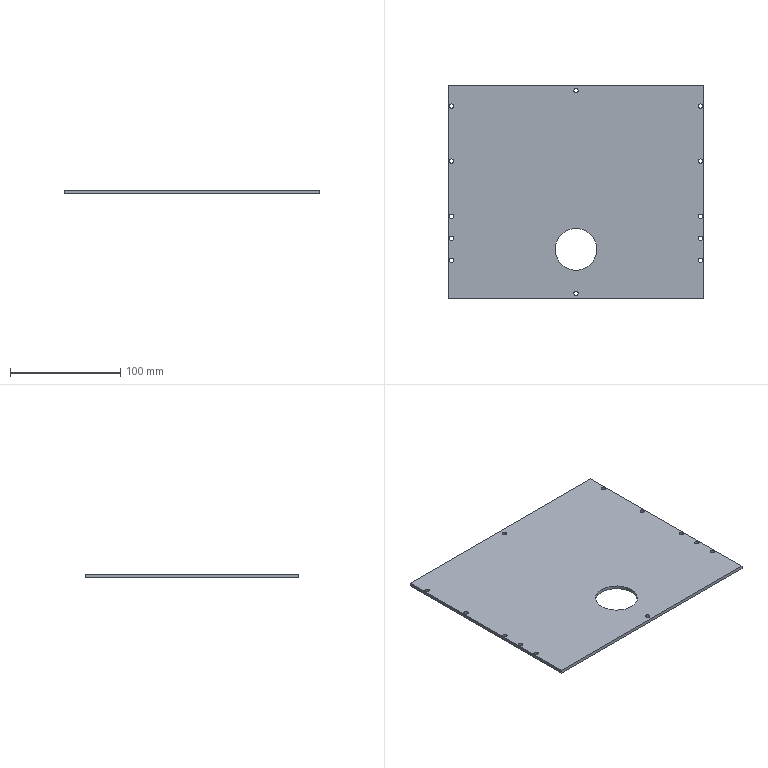Part | SolidWorks | features ICE 3, Extrusion 1, MirrorPattern 1 | 1 solid | 32 faces | box 232.3 x 194 x 3 mm | volume 131344 mm3 | cylinder 26 | plane 6 | commonest cylinder face diameters 4 x24 38 x2
STEP:
#1=CARTESIAN_POINT('',(115.15,-62.,0.));
#2=VERTEX_POINT('',#1);
#3=CARTESIAN_POINT('',(111.15,-62.,0.));
#4=VERTEX_POINT('',#3);
#5=CARTESIAN_POINT('',(113.15,-62.,0.));
#6=DIRECTION('',(0.,0.,-1.));
#7=DIRECTION('',(-1.,0.,0.));
#8=AXIS2_PLACEMENT_3D('',#5,#6,#7);
#9=CIRCLE('',#8,2.);
#10=EDGE_CURVE('',#2,#4,#9,.T.);
#11=ORIENTED_EDGE('',*,*,#10,.T.);
#12=CARTESIAN_POINT('',(111.15,-62.,3.));
#13=VERTEX_POINT('',#12);
#14=CARTESIAN_POINT('',(111.15,-62.,0.));
#15=DIRECTION('',(0.,0.,1.));
#16=VECTOR('',#15,1000.);
#17=LINE('',#14,#16);
#18=EDGE_CURVE('',#4,#13,#17,.T.);
#19=ORIENTED_EDGE('',*,*,#18,.T.);
#20=CARTESIAN_POINT('',(115.15,-62.,3.));
#21=VERTEX_POINT('',#20);
#22=CARTESIAN_POINT('',(113.15,-62.,3.));
#23=DIRECTION('',(0.,0.,-1.));
#24=DIRECTION('',(-1.,0.,0.));
#25=AXIS2_PLACEMENT_3D('',#22,#23,#24);
#26=CIRCLE('',#25,2.);
#27=EDGE_CURVE('',#21,#13,#26,.T.);
#28=ORIENTED_EDGE('',*,*,#27,.F.);
#29=CARTESIAN_POINT('',(115.15,-62.,0.));
#30=DIRECTION('',(0.,0.,1.));
#31=VECTOR('',#30,1000.);
#32=LINE('',#29,#31);
#33=EDGE_CURVE('',#2,#21,#32,.T.);
#34=ORIENTED_EDGE('',*,*,#33,.F.);
#35=EDGE_LOOP('',(#11,#19,#28,#34));
#36=FACE_OUTER_BOUND('',#35,.T.);
#37=CARTESIAN_POINT('',(113.15,-62.,0.));
#38=DIRECTION('',(0.,0.,1.));
#39=DIRECTION('',(1.,0.,0.));
#40=AXIS2_PLACEMENT_3D('',#37,#38,#39);
#41=CYLINDRICAL_SURFACE('',#40,2.);
#42=ADVANCED_FACE('',(#36),#41,.F.);
#43=CARTESIAN_POINT('',(115.15,-42.,0.));
#44=VERTEX_POINT('',#43);
#45=CARTESIAN_POINT('',(111.15,-42.,0.));
#46=VERTEX_POINT('',#45);
#47=CARTESIAN_POINT('',(113.15,-42.,0.));
#48=DIRECTION('',(0.,0.,-1.));
#49=DIRECTION('',(-1.,0.,0.));
#50=AXIS2_PLACEMENT_3D('',#47,#48,#49);
#51=CIRCLE('',#50,2.);
#52=EDGE_CURVE('',#44,#46,#51,.T.);
#53=ORIENTED_EDGE('',*,*,#52,.T.);
#54=CARTESIAN_POINT('',(111.15,-42.,3.));
#55=VERTEX_POINT('',#54);
#56=CARTESIAN_POINT('',(111.15,-42.,0.));
#57=DIRECTION('',(0.,0.,1.));
#58=VECTOR('',#57,1000.);
#59=LINE('',#56,#58);
#60=EDGE_CURVE('',#46,#55,#59,.T.);
#61=ORIENTED_EDGE('',*,*,#60,.T.);
#62=CARTESIAN_POINT('',(115.15,-42.,3.));
#63=VERTEX_POINT('',#62);
#64=CARTESIAN_POINT('',(113.15,-42.,3.));
#65=DIRECTION('',(0.,0.,-1.));
#66=DIRECTION('',(-1.,0.,0.));
#67=AXIS2_PLACEMENT_3D('',#64,#65,#66);
#68=CIRCLE('',#67,2.);
#69=EDGE_CURVE('',#63,#55,#68,.T.);
#70=ORIENTED_EDGE('',*,*,#69,.F.);
#71=CARTESIAN_POINT('',(115.15,-42.,0.));
#72=DIRECTION('',(0.,0.,1.));
#73=VECTOR('',#72,1000.);
#74=LINE('',#71,#73);
#75=EDGE_CURVE('',#44,#63,#74,.T.);
#76=ORIENTED_EDGE('',*,*,#75,.F.);
#77=EDGE_LOOP('',(#53,#61,#70,#76));
#78=FACE_OUTER_BOUND('',#77,.T.);
#79=CARTESIAN_POINT('',(113.15,-42.,0.));
#80=DIRECTION('',(0.,0.,1.));
#81=DIRECTION('',(1.,0.,0.));
#82=AXIS2_PLACEMENT_3D('',#79,#80,#81);
#83=CYLINDRICAL_SURFACE('',#82,2.);
#84=ADVANCED_FACE('',(#78),#83,.F.);
#85=CARTESIAN_POINT('',(115.15,-22.,0.));
#86=VERTEX_POINT('',#85);
#87=CARTESIAN_POINT('',(111.15,-22.,0.));
#88=VERTEX_POINT('',#87);
#89=CARTESIAN_POINT('',(113.15,-22.,0.));
#90=DIRECTION('',(0.,0.,-1.));
#91=DIRECTION('',(-1.,0.,0.));
#92=AXIS2_PLACEMENT_3D('',#89,#90,#91);
#93=CIRCLE('',#92,2.);
#94=EDGE_CURVE('',#86,#88,#93,.T.);
#95=ORIENTED_EDGE('',*,*,#94,.T.);
#96=CARTESIAN_POINT('',(111.15,-22.,3.));
#97=VERTEX_POINT('',#96);
#98=CARTESIAN_POINT('',(111.15,-22.,0.));
#99=DIRECTION('',(0.,0.,1.));
#100=VECTOR('',#99,1000.);
#101=LINE('',#98,#100);
#102=EDGE_CURVE('',#88,#97,#101,.T.);
#103=ORIENTED_EDGE('',*,*,#102,.T.);
#104=CARTESIAN_POINT('',(115.15,-22.,3.));
#105=VERTEX_POINT('',#104);
#106=CARTESIAN_POINT('',(113.15,-22.,3.));
#107=DIRECTION('',(0.,0.,-1.));
#108=DIRECTION('',(-1.,0.,0.));
#109=AXIS2_PLACEMENT_3D('',#106,#107,#108);
#110=CIRCLE('',#109,2.);
#111=EDGE_CURVE('',#105,#97,#110,.T.);
#112=ORIENTED_EDGE('',*,*,#111,.F.);
#113=CARTESIAN_POINT('',(115.15,-22.,0.));
#114=DIRECTION('',(0.,0.,1.));
#115=VECTOR('',#114,1000.);
#116=LINE('',#113,#115);
#117=EDGE_CURVE('',#86,#105,#116,.T.);
#118=ORIENTED_EDGE('',*,*,#117,.F.);
#119=EDGE_LOOP('',(#95,#103,#112,#118));
#120=FACE_OUTER_BOUND('',#119,.T.);
#121=CARTESIAN_POINT('',(113.15,-22.,0.));
#122=DIRECTION('',(0.,0.,1.));
#123=DIRECTION('',(1.,0.,0.));
#124=AXIS2_PLACEMENT_3D('',#121,#122,#123);
#125=CYLINDRICAL_SURFACE('',#124,2.);
#126=ADVANCED_FACE('',(#120),#125,.F.);
#127=CARTESIAN_POINT('',(115.15,28.,0.));
#128=VERTEX_POINT('',#127);
#129=CARTESIAN_POINT('',(111.15,28.,0.));
#130=VERTEX_POINT('',#129);
#131=CARTESIAN_POINT('',(113.15,28.,0.));
#132=DIRECTION('',(0.,0.,-1.));
#133=DIRECTION('',(-1.,0.,0.));
#134=AXIS2_PLACEMENT_3D('',#131,#132,#133);
#135=CIRCLE('',#134,2.);
#136=EDGE_CURVE('',#128,#130,#135,.T.);
#137=ORIENTED_EDGE('',*,*,#136,.T.);
#138=CARTESIAN_POINT('',(111.15,28.,3.));
#139=VERTEX_POINT('',#138);
#140=CARTESIAN_POINT('',(111.15,28.,0.));
#141=DIRECTION('',(0.,0.,1.));
#142=VECTOR('',#141,1000.);
#143=LINE('',#140,#142);
#144=EDGE_CURVE('',#130,#139,#143,.T.);
#145=ORIENTED_EDGE('',*,*,#144,.T.);
#146=CARTESIAN_POINT('',(115.15,28.,3.));
#147=VERTEX_POINT('',#146);
#148=CARTESIAN_POINT('',(113.15,28.,3.));
#149=DIRECTION('',(0.,0.,-1.));
#150=DIRECTION('',(-1.,0.,0.));
#151=AXIS2_PLACEMENT_3D('',#148,#149,#150);
#152=CIRCLE('',#151,2.);
#153=EDGE_CURVE('',#147,#139,#152,.T.);
#154=ORIENTED_EDGE('',*,*,#153,.F.);
#155=CARTESIAN_POINT('',(115.15,28.,0.));
#156=DIRECTION('',(0.,0.,1.));
#157=VECTOR('',#156,1000.);
#158=LINE('',#155,#157);
#159=EDGE_CURVE('',#128,#147,#158,.T.);
#160=ORIENTED_EDGE('',*,*,#159,.F.);
#161=EDGE_LOOP('',(#137,#145,#154,#160));
#162=FACE_OUTER_BOUND('',#161,.T.);
#163=CARTESIAN_POINT('',(113.15,28.,0.));
#164=DIRECTION('',(0.,0.,1.));
#165=DIRECTION('',(1.,0.,0.));
#166=AXIS2_PLACEMENT_3D('',#163,#164,#165);
#167=CYLINDRICAL_SURFACE('',#166,2.);
#168=ADVANCED_FACE('',(#162),#167,.F.);
#169=CARTESIAN_POINT('',(115.15,78.,0.));
#170=VERTEX_POINT('',#169);
#171=CARTESIAN_POINT('',(111.15,78.,0.));
#172=VERTEX_POINT('',#171);
#173=CARTESIAN_POINT('',(113.15,78.,0.));
#174=DIRECTION('',(0.,0.,-1.));
#175=DIRECTION('',(-1.,0.,0.));
#176=AXIS2_PLACEMENT_3D('',#173,#174,#175);
#177=CIRCLE('',#176,2.);
#178=EDGE_CURVE('',#170,#172,#177,.T.);
#179=ORIENTED_EDGE('',*,*,#178,.T.);
#180=CARTESIAN_POINT('',(111.15,78.,3.));
#181=VERTEX_POINT('',#180);
#182=CARTESIAN_POINT('',(111.15,78.,0.));
#183=DIRECTION('',(0.,0.,1.));
#184=VECTOR('',#183,1000.);
#185=LINE('',#182,#184);
#186=EDGE_CURVE('',#172,#181,#185,.T.);
#187=ORIENTED_EDGE('',*,*,#186,.T.);
#188=CARTESIAN_POINT('',(115.15,78.,3.));
#189=VERTEX_POINT('',#188);
#190=CARTESIAN_POINT('',(113.15,78.,3.));
#191=DIRECTION('',(0.,0.,-1.));
#192=DIRECTION('',(-1.,0.,0.));
#193=AXIS2_PLACEMENT_3D('',#190,#191,#192);
#194=CIRCLE('',#193,2.);
#195=EDGE_CURVE('',#189,#181,#194,.T.);
#196=ORIENTED_EDGE('',*,*,#195,.F.);
#197=CARTESIAN_POINT('',(115.15,78.,0.));
#198=DIRECTION('',(0.,0.,1.));
#199=VECTOR('',#198,1000.);
#200=LINE('',#197,#199);
#201=EDGE_CURVE('',#170,#189,#200,.T.);
#202=ORIENTED_EDGE('',*,*,#201,.F.);
#203=EDGE_LOOP('',(#179,#187,#196,#202));
#204=FACE_OUTER_BOUND('',#203,.T.);
#205=CARTESIAN_POINT('',(113.15,78.,0.));
#206=DIRECTION('',(0.,0.,1.));
#207=DIRECTION('',(1.,0.,0.));
#208=AXIS2_PLACEMENT_3D('',#205,#206,#207);
#209=CYLINDRICAL_SURFACE('',#208,2.);
#210=ADVANCED_FACE('',(#204),#209,.F.);
#211=CARTESIAN_POINT('',(-115.15,-62.,0.));
#212=VERTEX_POINT('',#211);
#213=CARTESIAN_POINT('',(-111.15,-62.,0.));
#214=VERTEX_POINT('',#213);
#215=CARTESIAN_POINT('',(-113.15,-62.,0.));
#216=DIRECTION('',(0.,0.,1.));
#217=DIRECTION('',(1.,0.,0.));
#218=AXIS2_PLACEMENT_3D('',#215,#216,#217);
#219=CIRCLE('',#218,2.);
#220=EDGE_CURVE('',#212,#214,#219,.T.);
#221=ORIENTED_EDGE('',*,*,#220,.F.);
#222=CARTESIAN_POINT('',(-115.15,-62.,3.));
#223=VERTEX_POINT('',#222);
#224=CARTESIAN_POINT('',(-115.15,-62.,0.));
#225=DIRECTION('',(0.,0.,1.));
#226=VECTOR('',#225,1000.);
#227=LINE('',#224,#226);
#228=EDGE_CURVE('',#212,#223,#227,.T.);
#229=ORIENTED_EDGE('',*,*,#228,.T.);
#230=CARTESIAN_POINT('',(-111.15,-62.,3.));
#231=VERTEX_POINT('',#230);
#232=CARTESIAN_POINT('',(-113.15,-62.,3.));
#233=DIRECTION('',(0.,0.,1.));
#234=DIRECTION('',(1.,0.,0.));
#235=AXIS2_PLACEMENT_3D('',#232,#233,#234);
#236=CIRCLE('',#235,2.);
#237=EDGE_CURVE('',#223,#231,#236,.T.);
#238=ORIENTED_EDGE('',*,*,#237,.T.);
#239=CARTESIAN_POINT('',(-111.15,-62.,0.));
#240=DIRECTION('',(0.,0.,1.));
#241=VECTOR('',#240,1000.);
#242=LINE('',#239,#241);
#243=EDGE_CURVE('',#214,#231,#242,.T.);
#244=ORIENTED_EDGE('',*,*,#243,.F.);
#245=EDGE_LOOP('',(#221,#229,#238,#244));
#246=FACE_OUTER_BOUND('',#245,.T.);
#247=CARTESIAN_POINT('',(-113.15,-62.,0.));
#248=DIRECTION('',(0.,0.,1.));
#249=DIRECTION('',(1.,0.,0.));
#250=AXIS2_PLACEMENT_3D('',#247,#248,#249);
#251=CYLINDRICAL_SURFACE('',#250,2.);
#252=ADVANCED_FACE('',(#246),#251,.F.);
#253=CARTESIAN_POINT('',(-115.15,-42.,0.));
#254=VERTEX_POINT('',#253);
#255=CARTESIAN_POINT('',(-111.15,-42.,0.));
#256=VERTEX_POINT('',#255);
#257=CARTESIAN_POINT('',(-113.15,-42.,0.));
#258=DIRECTION('',(0.,0.,1.));
#259=DIRECTION('',(1.,0.,0.));
#260=AXIS2_PLACEMENT_3D('',#257,#258,#259);
#261=CIRCLE('',#260,2.);
#262=EDGE_CURVE('',#254,#256,#261,.T.);
#263=ORIENTED_EDGE('',*,*,#262,.F.);
#264=CARTESIAN_POINT('',(-115.15,-42.,3.));
#265=VERTEX_POINT('',#264);
#266=CARTESIAN_POINT('',(-115.15,-42.,0.));
#267=DIRECTION('',(0.,0.,1.));
#268=VECTOR('',#267,1000.);
#269=LINE('',#266,#268);
#270=EDGE_CURVE('',#254,#265,#269,.T.);
#271=ORIENTED_EDGE('',*,*,#270,.T.);
#272=CARTESIAN_POINT('',(-111.15,-42.,3.));
#273=VERTEX_POINT('',#272);
#274=CARTESIAN_POINT('',(-113.15,-42.,3.));
#275=DIRECTION('',(0.,0.,1.));
#276=DIRECTION('',(1.,0.,0.));
#277=AXIS2_PLACEMENT_3D('',#274,#275,#276);
#278=CIRCLE('',#277,2.);
#279=EDGE_CURVE('',#265,#273,#278,.T.);
#280=ORIENTED_EDGE('',*,*,#279,.T.);
#281=CARTESIAN_POINT('',(-111.15,-42.,0.));
#282=DIRECTION('',(0.,0.,1.));
#283=VECTOR('',#282,1000.);
#284=LINE('',#281,#283);
#285=EDGE_CURVE('',#256,#273,#284,.T.);
#286=ORIENTED_EDGE('',*,*,#285,.F.);
#287=EDGE_LOOP('',(#263,#271,#280,#286));
#288=FACE_OUTER_BOUND('',#287,.T.);
#289=CARTESIAN_POINT('',(-113.15,-42.,0.));
#290=DIRECTION('',(0.,0.,1.));
#291=DIRECTION('',(1.,0.,0.));
#292=AXIS2_PLACEMENT_3D('',#289,#290,#291);
#293=CYLINDRICAL_SURFACE('',#292,2.);
#294=ADVANCED_FACE('',(#288),#293,.F.);
#295=CARTESIAN_POINT('',(-115.15,-22.,0.));
#296=VERTEX_POINT('',#295);
#297=CARTESIAN_POINT('',(-111.15,-22.,0.));
#298=VERTEX_POINT('',#297);
#299=CARTESIAN_POINT('',(-113.15,-22.,0.));
#300=DIRECTION('',(0.,0.,1.));
#301=DIRECTION('',(1.,0.,0.));
#302=AXIS2_PLACEMENT_3D('',#299,#300,#301);
#303=CIRCLE('',#302,2.);
#304=EDGE_CURVE('',#296,#298,#303,.T.);
#305=ORIENTED_EDGE('',*,*,#304,.F.);
#306=CARTESIAN_POINT('',(-115.15,-22.,3.));
#307=VERTEX_POINT('',#306);
#308=CARTESIAN_POINT('',(-115.15,-22.,0.));
#309=DIRECTION('',(0.,0.,1.));
#310=VECTOR('',#309,1000.);
#311=LINE('',#308,#310);
#312=EDGE_CURVE('',#296,#307,#311,.T.);
#313=ORIENTED_EDGE('',*,*,#312,.T.);
#314=CARTESIAN_POINT('',(-111.15,-22.,3.));
#315=VERTEX_POINT('',#314);
#316=CARTESIAN_POINT('',(-113.15,-22.,3.));
#317=DIRECTION('',(0.,0.,1.));
#318=DIRECTION('',(1.,0.,0.));
#319=AXIS2_PLACEMENT_3D('',#316,#317,#318);
#320=CIRCLE('',#319,2.);
#321=EDGE_CURVE('',#307,#315,#320,.T.);
#322=ORIENTED_EDGE('',*,*,#321,.T.);
#323=CARTESIAN_POINT('',(-111.15,-22.,0.));
#324=DIRECTION('',(0.,0.,1.));
#325=VECTOR('',#324,1000.);
#326=LINE('',#323,#325);
#327=EDGE_CURVE('',#298,#315,#326,.T.);
#328=ORIENTED_EDGE('',*,*,#327,.F.);
#329=EDGE_LOOP('',(#305,#313,#322,#328));
#330=FACE_OUTER_BOUND('',#329,.T.);
#331=CARTESIAN_POINT('',(-113.15,-22.,0.));
#332=DIRECTION('',(0.,0.,1.));
#333=DIRECTION('',(1.,0.,0.));
#334=AXIS2_PLACEMENT_3D('',#331,#332,#333);
#335=CYLINDRICAL_SURFACE('',#334,2.);
#336=ADVANCED_FACE('',(#330),#335,.F.);
#337=CARTESIAN_POINT('',(-115.15,28.,0.));
#338=VERTEX_POINT('',#337);
#339=CARTESIAN_POINT('',(-111.15,28.,0.));
#340=VERTEX_POINT('',#339);
#341=CARTESIAN_POINT('',(-113.15,28.,0.));
#342=DIRECTION('',(0.,0.,1.));
#343=DIRECTION('',(1.,0.,0.));
#344=AXIS2_PLACEMENT_3D('',#341,#342,#343);
#345=CIRCLE('',#344,2.);
#346=EDGE_CURVE('',#338,#340,#345,.T.);
#347=ORIENTED_EDGE('',*,*,#346,.F.);
#348=CARTESIAN_POINT('',(-115.15,28.,3.));
#349=VERTEX_POINT('',#348);
#350=CARTESIAN_POINT('',(-115.15,28.,0.));
#351=DIRECTION('',(0.,0.,1.));
#352=VECTOR('',#351,1000.);
#353=LINE('',#350,#352);
#354=EDGE_CURVE('',#338,#349,#353,.T.);
#355=ORIENTED_EDGE('',*,*,#354,.T.);
#356=CARTESIAN_POINT('',(-111.15,28.,3.));
#357=VERTEX_POINT('',#356);
#358=CARTESIAN_POINT('',(-113.15,28.,3.));
#359=DIRECTION('',(0.,0.,1.));
#360=DIRECTION('',(1.,0.,0.));
#361=AXIS2_PLACEMENT_3D('',#358,#359,#360);
#362=CIRCLE('',#361,2.);
#363=EDGE_CURVE('',#349,#357,#362,.T.);
#364=ORIENTED_EDGE('',*,*,#363,.T.);
#365=CARTESIAN_POINT('',(-111.15,28.,0.));
#366=DIRECTION('',(0.,0.,1.));
#367=VECTOR('',#366,1000.);
#368=LINE('',#365,#367);
#369=EDGE_CURVE('',#340,#357,#368,.T.);
#370=ORIENTED_EDGE('',*,*,#369,.F.);
#371=EDGE_LOOP('',(#347,#355,#364,#370));
#372=FACE_OUTER_BOUND('',#371,.T.);
#373=CARTESIAN_POINT('',(-113.15,28.,0.));
#374=DIRECTION('',(0.,0.,1.));
#375=DIRECTION('',(1.,0.,0.));
#376=AXIS2_PLACEMENT_3D('',#373,#374,#375);
#377=CYLINDRICAL_SURFACE('',#376,2.);
#378=ADVANCED_FACE('',(#372),#377,.F.);
#379=CARTESIAN_POINT('',(-115.15,78.,0.));
#380=VERTEX_POINT('',#379);
#381=CARTESIAN_POINT('',(-111.15,78.,0.));
#382=VERTEX_POINT('',#381);
#383=CARTESIAN_POINT('',(-113.15,78.,0.));
#384=DIRECTION('',(0.,0.,1.));
#385=DIRECTION('',(1.,0.,0.));
#386=AXIS2_PLACEMENT_3D('',#383,#384,#385);
#387=CIRCLE('',#386,2.);
#388=EDGE_CURVE('',#380,#382,#387,.T.);
#389=ORIENTED_EDGE('',*,*,#388,.F.);
#390=CARTESIAN_POINT('',(-115.15,78.,3.));
#391=VERTEX_POINT('',#390);
#392=CARTESIAN_POINT('',(-115.15,78.,0.));
#393=DIRECTION('',(0.,0.,1.));
#394=VECTOR('',#393,1000.);
#395=LINE('',#392,#394);
#396=EDGE_CURVE('',#380,#391,#395,.T.);
#397=ORIENTED_EDGE('',*,*,#396,.T.);
#398=CARTESIAN_POINT('',(-111.15,78.,3.));
#399=VERTEX_POINT('',#398);
#400=CARTESIAN_POINT('',(-113.15,78.,3.));
#401=DIRECTION('',(0.,0.,1.));
#402=DIRECTION('',(1.,0.,0.));
#403=AXIS2_PLACEMENT_3D('',#400,#401,#402);
#404=CIRCLE('',#403,2.);
#405=EDGE_CURVE('',#391,#399,#404,.T.);
#406=ORIENTED_EDGE('',*,*,#405,.T.);
#407=CARTESIAN_POINT('',(-111.15,78.,0.));
#408=DIRECTION('',(0.,0.,1.));
#409=VECTOR('',#408,1000.);
#410=LINE('',#407,#409);
#411=EDGE_CURVE('',#382,#399,#410,.T.);
#412=ORIENTED_EDGE('',*,*,#411,.F.);
#413=EDGE_LOOP('',(#389,#397,#406,#412));
#414=FACE_OUTER_BOUND('',#413,.T.);
#415=CARTESIAN_POINT('',(-113.15,78.,0.));
#416=DIRECTION('',(0.,0.,1.));
#417=DIRECTION('',(1.,0.,0.));
#418=AXIS2_PLACEMENT_3D('',#415,#416,#417);
#419=CYLINDRICAL_SURFACE('',#418,2.);
#420=ADVANCED_FACE('',(#414),#419,.F.);
#421=CARTESIAN_POINT('',(-2.,-92.,0.));
#422=VERTEX_POINT('',#421);
#423=CARTESIAN_POINT('',(2.,-92.,0.));
#424=VERTEX_POINT('',#423);
#425=CARTESIAN_POINT('',(0.,-92.,0.));
#426=DIRECTION('',(0.,0.,1.));
#427=DIRECTION('',(1.,0.,0.));
#428=AXIS2_PLACEMENT_3D('',#425,#426,#427);
#429=CIRCLE('',#428,2.);
#430=EDGE_CURVE('',#422,#424,#429,.T.);
#431=ORIENTED_EDGE('',*,*,#430,.F.);
#432=CARTESIAN_POINT('',(-2.,-92.,3.));
#433=VERTEX_POINT('',#432);
#434=CARTESIAN_POINT('',(-2.,-92.,-1.));
#435=DIRECTION('',(0.,0.,1.));
#436=VECTOR('',#435,1000.);
#437=LINE('',#434,#436);
#438=EDGE_CURVE('',#422,#433,#437,.T.);
#439=ORIENTED_EDGE('',*,*,#438,.T.);
#440=CARTESIAN_POINT('',(2.,-92.,3.));
#441=VERTEX_POINT('',#440);
#442=CARTESIAN_POINT('',(0.,-92.,3.));
#443=DIRECTION('',(0.,0.,1.));
#444=DIRECTION('',(-1.,0.,0.));
#445=AXIS2_PLACEMENT_3D('',#442,#443,#444);
#446=CIRCLE('',#445,2.);
#447=EDGE_CURVE('',#433,#441,#446,.T.);
#448=ORIENTED_EDGE('',*,*,#447,.T.);
#449=CARTESIAN_POINT('',(2.,-92.,-1.));
#450=DIRECTION('',(0.,0.,1.));
#451=VECTOR('',#450,1000.);
#452=LINE('',#449,#451);
#453=EDGE_CURVE('',#424,#441,#452,.T.);
#454=ORIENTED_EDGE('',*,*,#453,.F.);
#455=EDGE_LOOP('',(#431,#439,#448,#454));
#456=FACE_OUTER_BOUND('',#455,.T.);
#457=CARTESIAN_POINT('',(0.,-92.,-1.));
#458=DIRECTION('',(0.,0.,1.));
#459=DIRECTION('',(1.,0.,0.));
#460=AXIS2_PLACEMENT_3D('',#457,#458,#459);
#461=CYLINDRICAL_SURFACE('',#460,2.);
#462=ADVANCED_FACE('',(#456),#461,.F.);
#463=CARTESIAN_POINT('',(-2.,92.,0.));
#464=VERTEX_POINT('',#463);
#465=CARTESIAN_POINT('',(2.,92.,0.));
#466=VERTEX_POINT('',#465);
#467=CARTESIAN_POINT('',(0.,92.,0.));
#468=DIRECTION('',(0.,0.,1.));
#469=DIRECTION('',(1.,0.,0.));
#470=AXIS2_PLACEMENT_3D('',#467,#468,#469);
#471=CIRCLE('',#470,2.);
#472=EDGE_CURVE('',#464,#466,#471,.T.);
#473=ORIENTED_EDGE('',*,*,#472,.F.);
#474=CARTESIAN_POINT('',(-2.,92.,3.));
#475=VERTEX_POINT('',#474);
#476=CARTESIAN_POINT('',(-2.,92.,-1.));
#477=DIRECTION('',(0.,0.,1.));
#478=VECTOR('',#477,1000.);
#479=LINE('',#476,#478);
#480=EDGE_CURVE('',#464,#475,#479,.T.);
#481=ORIENTED_EDGE('',*,*,#480,.T.);
#482=CARTESIAN_POINT('',(2.,92.,3.));
#483=VERTEX_POINT('',#482);
#484=CARTESIAN_POINT('',(0.,92.,3.));
#485=DIRECTION('',(0.,0.,1.));
#486=DIRECTION('',(1.,0.,0.));
#487=AXIS2_PLACEMENT_3D('',#484,#485,#486);
#488=CIRCLE('',#487,2.);
#489=EDGE_CURVE('',#475,#483,#488,.T.);
#490=ORIENTED_EDGE('',*,*,#489,.T.);
#491=CARTESIAN_POINT('',(2.,92.,-1.));
#492=DIRECTION('',(0.,0.,1.));
#493=VECTOR('',#492,1000.);
#494=LINE('',#491,#493);
#495=EDGE_CURVE('',#466,#483,#494,.T.);
#496=ORIENTED_EDGE('',*,*,#495,.F.);
#497=EDGE_LOOP('',(#473,#481,#490,#496));
#498=FACE_OUTER_BOUND('',#497,.T.);
#499=CARTESIAN_POINT('',(0.,92.,-1.));
#500=DIRECTION('',(0.,0.,1.));
#501=DIRECTION('',(1.,0.,0.));
#502=AXIS2_PLACEMENT_3D('',#499,#500,#501);
#503=CYLINDRICAL_SURFACE('',#502,2.);
#504=ADVANCED_FACE('',(#498),#503,.F.);
#505=CARTESIAN_POINT('',(-19.,-52.,0.));
#506=VERTEX_POINT('',#505);
#507=CARTESIAN_POINT('',(19.,-52.,0.));
#508=VERTEX_POINT('',#507);
#509=CARTESIAN_POINT('',(0.,-52.,0.));
#510=DIRECTION('',(0.,0.,1.));
#511=DIRECTION('',(1.,0.,0.));
#512=AXIS2_PLACEMENT_3D('',#509,#510,#511);
#513=CIRCLE('',#512,19.);
#514=EDGE_CURVE('',#506,#508,#513,.T.);
#515=ORIENTED_EDGE('',*,*,#514,.F.);
#516=CARTESIAN_POINT('',(-19.,-52.,3.));
#517=VERTEX_POINT('',#516);
#518=CARTESIAN_POINT('',(-19.,-52.,0.));
#519=DIRECTION('',(0.,0.,1.));
#520=VECTOR('',#519,1000.);
#521=LINE('',#518,#520);
#522=EDGE_CURVE('',#506,#517,#521,.T.);
#523=ORIENTED_EDGE('',*,*,#522,.T.);
#524=CARTESIAN_POINT('',(19.,-52.,3.));
#525=VERTEX_POINT('',#524);
#526=CARTESIAN_POINT('',(0.,-52.,3.));
#527=DIRECTION('',(0.,0.,1.));
#528=DIRECTION('',(1.,0.,0.));
#529=AXIS2_PLACEMENT_3D('',#526,#527,#528);
#530=CIRCLE('',#529,19.);
#531=EDGE_CURVE('',#517,#525,#530,.T.);
#532=ORIENTED_EDGE('',*,*,#531,.T.);
#533=CARTESIAN_POINT('',(19.,-52.,0.));
#534=DIRECTION('',(0.,0.,1.));
#535=VECTOR('',#534,1000.);
#536=LINE('',#533,#535);
#537=EDGE_CURVE('',#508,#525,#536,.T.);
#538=ORIENTED_EDGE('',*,*,#537,.F.);
#539=EDGE_LOOP('',(#515,#523,#532,#538));
#540=FACE_OUTER_BOUND('',#539,.T.);
#541=CARTESIAN_POINT('',(0.,-52.,0.));
#542=DIRECTION('',(0.,0.,1.));
#543=DIRECTION('',(1.,0.,0.));
#544=AXIS2_PLACEMENT_3D('',#541,#542,#543);
#545=CYLINDRICAL_SURFACE('',#544,19.);
#546=ADVANCED_FACE('',(#540),#545,.F.);
#547=ORIENTED_EDGE('',*,*,#69,.T.);
#548=CARTESIAN_POINT('',(113.15,-42.,3.));
#549=DIRECTION('',(0.,0.,-1.));
#550=DIRECTION('',(-1.,0.,0.));
#551=AXIS2_PLACEMENT_3D('',#548,#549,#550);
#552=CIRCLE('',#551,2.);
#553=EDGE_CURVE('',#55,#63,#552,.T.);
#554=ORIENTED_EDGE('',*,*,#553,.T.);
#555=EDGE_LOOP('',(#547,#554));
#556=FACE_BOUND('',#555,.T.);
#557=ORIENTED_EDGE('',*,*,#153,.T.);
#558=CARTESIAN_POINT('',(113.15,28.,3.));
#559=DIRECTION('',(0.,0.,-1.));
#560=DIRECTION('',(-1.,0.,0.));
#561=AXIS2_PLACEMENT_3D('',#558,#559,#560);
#562=CIRCLE('',#561,2.);
#563=EDGE_CURVE('',#139,#147,#562,.T.);
#564=ORIENTED_EDGE('',*,*,#563,.T.);
#565=EDGE_LOOP('',(#557,#564));
#566=FACE_BOUND('',#565,.T.);
#567=CARTESIAN_POINT('',(116.15,-97.,3.));
#568=VERTEX_POINT('',#567);
#569=CARTESIAN_POINT('',(116.15,97.,3.));
#570=VERTEX_POINT('',#569);
#571=CARTESIAN_POINT('',(116.15,97.,3.));
#572=DIRECTION('',(0.,1.,0.));
#573=VECTOR('',#572,1000.);
#574=LINE('',#571,#573);
#575=EDGE_CURVE('',#568,#570,#574,.T.);
#576=ORIENTED_EDGE('',*,*,#575,.T.);
#577=CARTESIAN_POINT('',(-116.15,97.,3.));
#578=VERTEX_POINT('',#577);
#579=CARTESIAN_POINT('',(-116.15,97.,3.));
#580=DIRECTION('',(-1.,0.,0.));
#581=VECTOR('',#580,1000.);
#582=LINE('',#579,#581);
#583=EDGE_CURVE('',#570,#578,#582,.T.);
#584=ORIENTED_EDGE('',*,*,#583,.T.);
#585=CARTESIAN_POINT('',(-116.15,-97.,3.));
#586=VERTEX_POINT('',#585);
#587=CARTESIAN_POINT('',(-116.15,97.,3.));
#588=DIRECTION('',(0.,-1.,0.));
#589=VECTOR('',#588,1000.);
#590=LINE('',#587,#589);
#591=EDGE_CURVE('',#578,#586,#590,.T.);
#592=ORIENTED_EDGE('',*,*,#591,.T.);
#593=CARTESIAN_POINT('',(-116.15,-97.,3.));
#594=DIRECTION('',(1.,0.,0.));
#595=VECTOR('',#594,1000.);
#596=LINE('',#593,#595);
#597=EDGE_CURVE('',#586,#568,#596,.T.);
#598=ORIENTED_EDGE('',*,*,#597,.T.);
#599=EDGE_LOOP('',(#576,#584,#592,#598));
#600=FACE_OUTER_BOUND('',#599,.T.);
#601=CARTESIAN_POINT('',(0.,-52.,3.));
#602=DIRECTION('',(0.,0.,1.));
#603=DIRECTION('',(1.,0.,0.));
#604=AXIS2_PLACEMENT_3D('',#601,#602,#603);
#605=CIRCLE('',#604,19.);
#606=EDGE_CURVE('',#525,#517,#605,.T.);
#607=ORIENTED_EDGE('',*,*,#606,.F.);
#608=ORIENTED_EDGE('',*,*,#531,.F.);
#609=EDGE_LOOP('',(#607,#608));
#610=FACE_BOUND('',#609,.T.);
#611=CARTESIAN_POINT('',(0.,92.,3.));
#612=DIRECTION('',(0.,0.,1.));
#613=DIRECTION('',(1.,0.,0.));
#614=AXIS2_PLACEMENT_3D('',#611,#612,#613);
#615=CIRCLE('',#614,2.);
#616=EDGE_CURVE('',#483,#475,#615,.T.);
#617=ORIENTED_EDGE('',*,*,#616,.F.);
#618=ORIENTED_EDGE('',*,*,#489,.F.);
#619=EDGE_LOOP('',(#617,#618));
#620=FACE_BOUND('',#619,.T.);
#621=CARTESIAN_POINT('',(0.,-92.,3.));
#622=DIRECTION('',(0.,0.,1.));
#623=DIRECTION('',(-1.,0.,0.));
#624=AXIS2_PLACEMENT_3D('',#621,#622,#623);
#625=CIRCLE('',#624,2.);
#626=EDGE_CURVE('',#441,#433,#625,.T.);
#627=ORIENTED_EDGE('',*,*,#626,.F.);
#628=ORIENTED_EDGE('',*,*,#447,.F.);
#629=EDGE_LOOP('',(#627,#628));
#630=FACE_BOUND('',#629,.T.);
#631=CARTESIAN_POINT('',(-113.15,78.,3.));
#632=DIRECTION('',(0.,0.,1.));
#633=DIRECTION('',(1.,0.,0.));
#634=AXIS2_PLACEMENT_3D('',#631,#632,#633);
#635=CIRCLE('',#634,2.);
#636=EDGE_CURVE('',#399,#391,#635,.T.);
#637=ORIENTED_EDGE('',*,*,#636,.F.);
#638=ORIENTED_EDGE('',*,*,#405,.F.);
#639=EDGE_LOOP('',(#637,#638));
#640=FACE_BOUND('',#639,.T.);
#641=CARTESIAN_POINT('',(-113.15,28.,3.));
#642=DIRECTION('',(0.,0.,1.));
#643=DIRECTION('',(1.,0.,0.));
#644=AXIS2_PLACEMENT_3D('',#641,#642,#643);
#645=CIRCLE('',#644,2.);
#646=EDGE_CURVE('',#357,#349,#645,.T.);
#647=ORIENTED_EDGE('',*,*,#646,.F.);
#648=ORIENTED_EDGE('',*,*,#363,.F.);
#649=EDGE_LOOP('',(#647,#648));
#650=FACE_BOUND('',#649,.T.);
#651=CARTESIAN_POINT('',(-113.15,-22.,3.));
#652=DIRECTION('',(0.,0.,1.));
#653=DIRECTION('',(1.,0.,0.));
#654=AXIS2_PLACEMENT_3D('',#651,#652,#653);
#655=CIRCLE('',#654,2.);
#656=EDGE_CURVE('',#315,#307,#655,.T.);
#657=ORIENTED_EDGE('',*,*,#656,.F.);
#658=ORIENTED_EDGE('',*,*,#321,.F.);
#659=EDGE_LOOP('',(#657,#658));
#660=FACE_BOUND('',#659,.T.);
#661=CARTESIAN_POINT('',(-113.15,-42.,3.));
#662=DIRECTION('',(0.,0.,1.));
#663=DIRECTION('',(1.,0.,0.));
#664=AXIS2_PLACEMENT_3D('',#661,#662,#663);
#665=CIRCLE('',#664,2.);
#666=EDGE_CURVE('',#273,#265,#665,.T.);
#667=ORIENTED_EDGE('',*,*,#666,.F.);
#668=ORIENTED_EDGE('',*,*,#279,.F.);
#669=EDGE_LOOP('',(#667,#668));
#670=FACE_BOUND('',#669,.T.);
#671=CARTESIAN_POINT('',(-113.15,-62.,3.));
#672=DIRECTION('',(0.,0.,1.));
#673=DIRECTION('',(1.,0.,0.));
#674=AXIS2_PLACEMENT_3D('',#671,#672,#673);
#675=CIRCLE('',#674,2.);
#676=EDGE_CURVE('',#231,#223,#675,.T.);
#677=ORIENTED_EDGE('',*,*,#676,.F.);
#678=ORIENTED_EDGE('',*,*,#237,.F.);
#679=EDGE_LOOP('',(#677,#678));
#680=FACE_BOUND('',#679,.T.);
#681=ORIENTED_EDGE('',*,*,#195,.T.);
#682=CARTESIAN_POINT('',(113.15,78.,3.));
#683=DIRECTION('',(0.,0.,-1.));
#684=DIRECTION('',(-1.,0.,0.));
#685=AXIS2_PLACEMENT_3D('',#682,#683,#684);
#686=CIRCLE('',#685,2.);
#687=EDGE_CURVE('',#181,#189,#686,.T.);
#688=ORIENTED_EDGE('',*,*,#687,.T.);
#689=EDGE_LOOP('',(#681,#688));
#690=FACE_BOUND('',#689,.T.);
#691=ORIENTED_EDGE('',*,*,#111,.T.);
#692=CARTESIAN_POINT('',(113.15,-22.,3.));
#693=DIRECTION('',(0.,0.,-1.));
#694=DIRECTION('',(-1.,0.,0.));
#695=AXIS2_PLACEMENT_3D('',#692,#693,#694);
#696=CIRCLE('',#695,2.);
#697=EDGE_CURVE('',#97,#105,#696,.T.);
#698=ORIENTED_EDGE('',*,*,#697,.T.);
#699=EDGE_LOOP('',(#691,#698));
#700=FACE_BOUND('',#699,.T.);
#701=ORIENTED_EDGE('',*,*,#27,.T.);
#702=CARTESIAN_POINT('',(113.15,-62.,3.));
#703=DIRECTION('',(0.,0.,-1.));
#704=DIRECTION('',(-1.,0.,0.));
#705=AXIS2_PLACEMENT_3D('',#702,#703,#704);
#706=CIRCLE('',#705,2.);
#707=EDGE_CURVE('',#13,#21,#706,.T.);
#708=ORIENTED_EDGE('',*,*,#707,.T.);
#709=EDGE_LOOP('',(#701,#708));
#710=FACE_BOUND('',#709,.T.);
#711=CARTESIAN_POINT('',(0.,0.,3.));
#712=DIRECTION('',(0.,0.,1.));
#713=DIRECTION('',(1.,0.,0.));
#714=AXIS2_PLACEMENT_3D('',#711,#712,#713);
#715=PLANE('',#714);
#716=ADVANCED_FACE('',(#556,#566,#600,#610,#620,#630,#640,#650,#660,#670,#680,#690,#700,#710),#715,.T.);
#717=ORIENTED_EDGE('',*,*,#52,.F.);
#718=CARTESIAN_POINT('',(113.15,-42.,0.));
#719=DIRECTION('',(0.,0.,-1.));
#720=DIRECTION('',(-1.,0.,0.));
#721=AXIS2_PLACEMENT_3D('',#718,#719,#720);
#722=CIRCLE('',#721,2.);
#723=EDGE_CURVE('',#46,#44,#722,.T.);
#724=ORIENTED_EDGE('',*,*,#723,.F.);
#725=EDGE_LOOP('',(#717,#724));
#726=FACE_BOUND('',#725,.T.);
#727=ORIENTED_EDGE('',*,*,#136,.F.);
#728=CARTESIAN_POINT('',(113.15,28.,0.));
#729=DIRECTION('',(0.,0.,-1.));
#730=DIRECTION('',(-1.,0.,0.));
#731=AXIS2_PLACEMENT_3D('',#728,#729,#730);
#732=CIRCLE('',#731,2.);
#733=EDGE_CURVE('',#130,#128,#732,.T.);
#734=ORIENTED_EDGE('',*,*,#733,.F.);
#735=EDGE_LOOP('',(#727,#734));
#736=FACE_BOUND('',#735,.T.);
#737=CARTESIAN_POINT('',(116.15,-97.,0.));
#738=VERTEX_POINT('',#737);
#739=CARTESIAN_POINT('',(116.15,97.,0.));
#740=VERTEX_POINT('',#739);
#741=CARTESIAN_POINT('',(116.15,97.,0.));
#742=DIRECTION('',(0.,1.,0.));
#743=VECTOR('',#742,1000.);
#744=LINE('',#741,#743);
#745=EDGE_CURVE('',#738,#740,#744,.T.);
#746=ORIENTED_EDGE('',*,*,#745,.F.);
#747=CARTESIAN_POINT('',(-116.15,-97.,0.));
#748=VERTEX_POINT('',#747);
#749=CARTESIAN_POINT('',(-116.15,-97.,0.));
#750=DIRECTION('',(1.,0.,0.));
#751=VECTOR('',#750,1000.);
#752=LINE('',#749,#751);
#753=EDGE_CURVE('',#748,#738,#752,.T.);
#754=ORIENTED_EDGE('',*,*,#753,.F.);
#755=CARTESIAN_POINT('',(-116.15,97.,0.));
#756=VERTEX_POINT('',#755);
#757=CARTESIAN_POINT('',(-116.15,97.,0.));
#758=DIRECTION('',(0.,-1.,0.));
#759=VECTOR('',#758,1000.);
#760=LINE('',#757,#759);
#761=EDGE_CURVE('',#756,#748,#760,.T.);
#762=ORIENTED_EDGE('',*,*,#761,.F.);
#763=CARTESIAN_POINT('',(-116.15,97.,0.));
#764=DIRECTION('',(-1.,0.,0.));
#765=VECTOR('',#764,1000.);
#766=LINE('',#763,#765);
#767=EDGE_CURVE('',#740,#756,#766,.T.);
#768=ORIENTED_EDGE('',*,*,#767,.F.);
#769=EDGE_LOOP('',(#746,#754,#762,#768));
#770=FACE_OUTER_BOUND('',#769,.T.);
#771=CARTESIAN_POINT('',(0.,-52.,0.));
#772=DIRECTION('',(0.,0.,1.));
#773=DIRECTION('',(1.,0.,0.));
#774=AXIS2_PLACEMENT_3D('',#771,#772,#773);
#775=CIRCLE('',#774,19.);
#776=EDGE_CURVE('',#508,#506,#775,.T.);
#777=ORIENTED_EDGE('',*,*,#776,.T.);
#778=ORIENTED_EDGE('',*,*,#514,.T.);
#779=EDGE_LOOP('',(#777,#778));
#780=FACE_BOUND('',#779,.T.);
#781=CARTESIAN_POINT('',(0.,92.,0.));
#782=DIRECTION('',(0.,0.,1.));
#783=DIRECTION('',(1.,0.,0.));
#784=AXIS2_PLACEMENT_3D('',#781,#782,#783);
#785=CIRCLE('',#784,2.);
#786=EDGE_CURVE('',#466,#464,#785,.T.);
#787=ORIENTED_EDGE('',*,*,#786,.T.);
#788=ORIENTED_EDGE('',*,*,#472,.T.);
#789=EDGE_LOOP('',(#787,#788));
#790=FACE_BOUND('',#789,.T.);
#791=CARTESIAN_POINT('',(0.,-92.,0.));
#792=DIRECTION('',(0.,0.,1.));
#793=DIRECTION('',(1.,0.,0.));
#794=AXIS2_PLACEMENT_3D('',#791,#792,#793);
#795=CIRCLE('',#794,2.);
#796=EDGE_CURVE('',#424,#422,#795,.T.);
#797=ORIENTED_EDGE('',*,*,#796,.T.);
#798=ORIENTED_EDGE('',*,*,#430,.T.);
#799=EDGE_LOOP('',(#797,#798));
#800=FACE_BOUND('',#799,.T.);
#801=CARTESIAN_POINT('',(-113.15,78.,0.));
#802=DIRECTION('',(0.,0.,1.));
#803=DIRECTION('',(1.,0.,0.));
#804=AXIS2_PLACEMENT_3D('',#801,#802,#803);
#805=CIRCLE('',#804,2.);
#806=EDGE_CURVE('',#382,#380,#805,.T.);
#807=ORIENTED_EDGE('',*,*,#806,.T.);
#808=ORIENTED_EDGE('',*,*,#388,.T.);
#809=EDGE_LOOP('',(#807,#808));
#810=FACE_BOUND('',#809,.T.);
#811=CARTESIAN_POINT('',(-113.15,28.,0.));
#812=DIRECTION('',(0.,0.,1.));
#813=DIRECTION('',(1.,0.,0.));
#814=AXIS2_PLACEMENT_3D('',#811,#812,#813);
#815=CIRCLE('',#814,2.);
#816=EDGE_CURVE('',#340,#338,#815,.T.);
#817=ORIENTED_EDGE('',*,*,#816,.T.);
#818=ORIENTED_EDGE('',*,*,#346,.T.);
#819=EDGE_LOOP('',(#817,#818));
#820=FACE_BOUND('',#819,.T.);
#821=CARTESIAN_POINT('',(-113.15,-22.,0.));
#822=DIRECTION('',(0.,0.,1.));
#823=DIRECTION('',(1.,0.,0.));
#824=AXIS2_PLACEMENT_3D('',#821,#822,#823);
#825=CIRCLE('',#824,2.);
#826=EDGE_CURVE('',#298,#296,#825,.T.);
#827=ORIENTED_EDGE('',*,*,#826,.T.);
#828=ORIENTED_EDGE('',*,*,#304,.T.);
#829=EDGE_LOOP('',(#827,#828));
#830=FACE_BOUND('',#829,.T.);
#831=CARTESIAN_POINT('',(-113.15,-42.,0.));
#832=DIRECTION('',(0.,0.,1.));
#833=DIRECTION('',(1.,0.,0.));
#834=AXIS2_PLACEMENT_3D('',#831,#832,#833);
#835=CIRCLE('',#834,2.);
#836=EDGE_CURVE('',#256,#254,#835,.T.);
#837=ORIENTED_EDGE('',*,*,#836,.T.);
#838=ORIENTED_EDGE('',*,*,#262,.T.);
#839=EDGE_LOOP('',(#837,#838));
#840=FACE_BOUND('',#839,.T.);
#841=CARTESIAN_POINT('',(-113.15,-62.,0.));
#842=DIRECTION('',(0.,0.,1.));
#843=DIRECTION('',(1.,0.,0.));
#844=AXIS2_PLACEMENT_3D('',#841,#842,#843);
#845=CIRCLE('',#844,2.);
#846=EDGE_CURVE('',#214,#212,#845,.T.);
#847=ORIENTED_EDGE('',*,*,#846,.T.);
#848=ORIENTED_EDGE('',*,*,#220,.T.);
#849=EDGE_LOOP('',(#847,#848));
#850=FACE_BOUND('',#849,.T.);
#851=ORIENTED_EDGE('',*,*,#178,.F.);
#852=CARTESIAN_POINT('',(113.15,78.,0.));
#853=DIRECTION('',(0.,0.,-1.));
#854=DIRECTION('',(-1.,0.,0.));
#855=AXIS2_PLACEMENT_3D('',#852,#853,#854);
#856=CIRCLE('',#855,2.);
#857=EDGE_CURVE('',#172,#170,#856,.T.);
#858=ORIENTED_EDGE('',*,*,#857,.F.);
#859=EDGE_LOOP('',(#851,#858));
#860=FACE_BOUND('',#859,.T.);
#861=ORIENTED_EDGE('',*,*,#94,.F.);
#862=CARTESIAN_POINT('',(113.15,-22.,0.));
#863=DIRECTION('',(0.,0.,-1.));
#864=DIRECTION('',(-1.,0.,0.));
#865=AXIS2_PLACEMENT_3D('',#862,#863,#864);
#866=CIRCLE('',#865,2.);
#867=EDGE_CURVE('',#88,#86,#866,.T.);
#868=ORIENTED_EDGE('',*,*,#867,.F.);
#869=EDGE_LOOP('',(#861,#868));
#870=FACE_BOUND('',#869,.T.);
#871=ORIENTED_EDGE('',*,*,#10,.F.);
#872=CARTESIAN_POINT('',(113.15,-62.,0.));
#873=DIRECTION('',(0.,0.,-1.));
#874=DIRECTION('',(-1.,0.,0.));
#875=AXIS2_PLACEMENT_3D('',#872,#873,#874);
#876=CIRCLE('',#875,2.);
#877=EDGE_CURVE('',#4,#2,#876,.T.);
#878=ORIENTED_EDGE('',*,*,#877,.F.);
#879=EDGE_LOOP('',(#871,#878));
#880=FACE_BOUND('',#879,.T.);
#881=CARTESIAN_POINT('',(0.,0.,0.));
#882=DIRECTION('',(0.,0.,1.));
#883=DIRECTION('',(1.,0.,0.));
#884=AXIS2_PLACEMENT_3D('',#881,#882,#883);
#885=PLANE('',#884);
#886=ADVANCED_FACE('',(#726,#736,#770,#780,#790,#800,#810,#820,#830,#840,#850,#860,#870,#880),#885,.F.);
#887=ORIENTED_EDGE('',*,*,#745,.T.);
#888=CARTESIAN_POINT('',(116.15,97.,3.));
#889=DIRECTION('',(0.,0.,-1.));
#890=VECTOR('',#889,1000.);
#891=LINE('',#888,#890);
#892=EDGE_CURVE('',#570,#740,#891,.T.);
#893=ORIENTED_EDGE('',*,*,#892,.F.);
#894=ORIENTED_EDGE('',*,*,#575,.F.);
#895=CARTESIAN_POINT('',(116.15,-97.,3.));
#896=DIRECTION('',(0.,0.,-1.));
#897=VECTOR('',#896,1000.);
#898=LINE('',#895,#897);
#899=EDGE_CURVE('',#568,#738,#898,.T.);
#900=ORIENTED_EDGE('',*,*,#899,.T.);
#901=EDGE_LOOP('',(#887,#893,#894,#900));
#902=FACE_OUTER_BOUND('',#901,.T.);
#903=CARTESIAN_POINT('',(116.15,97.,3.));
#904=DIRECTION('',(-1.,0.,0.));
#905=DIRECTION('',(0.,0.,1.));
#906=AXIS2_PLACEMENT_3D('',#903,#904,#905);
#907=PLANE('',#906);
#908=ADVANCED_FACE('',(#902),#907,.F.);
#909=ORIENTED_EDGE('',*,*,#767,.T.);
#910=CARTESIAN_POINT('',(-116.15,97.,3.));
#911=DIRECTION('',(0.,0.,-1.));
#912=VECTOR('',#911,1000.);
#913=LINE('',#910,#912);
#914=EDGE_CURVE('',#578,#756,#913,.T.);
#915=ORIENTED_EDGE('',*,*,#914,.F.);
#916=ORIENTED_EDGE('',*,*,#583,.F.);
#917=ORIENTED_EDGE('',*,*,#892,.T.);
#918=EDGE_LOOP('',(#909,#915,#916,#917));
#919=FACE_OUTER_BOUND('',#918,.T.);
#920=CARTESIAN_POINT('',(-116.15,97.,3.));
#921=DIRECTION('',(0.,-1.,0.));
#922=DIRECTION('',(0.,0.,-1.));
#923=AXIS2_PLACEMENT_3D('',#920,#921,#922);
#924=PLANE('',#923);
#925=ADVANCED_FACE('',(#919),#924,.F.);
#926=ORIENTED_EDGE('',*,*,#761,.T.);
#927=CARTESIAN_POINT('',(-116.15,-97.,3.));
#928=DIRECTION('',(0.,0.,-1.));
#929=VECTOR('',#928,1000.);
#930=LINE('',#927,#929);
#931=EDGE_CURVE('',#586,#748,#930,.T.);
#932=ORIENTED_EDGE('',*,*,#931,.F.);
#933=ORIENTED_EDGE('',*,*,#591,.F.);
#934=ORIENTED_EDGE('',*,*,#914,.T.);
#935=EDGE_LOOP('',(#926,#932,#933,#934));
#936=FACE_OUTER_BOUND('',#935,.T.);
#937=CARTESIAN_POINT('',(-116.15,97.,3.));
#938=DIRECTION('',(1.,0.,0.));
#939=DIRECTION('',(0.,1.,0.));
#940=AXIS2_PLACEMENT_3D('',#937,#938,#939);
#941=PLANE('',#940);
#942=ADVANCED_FACE('',(#936),#941,.F.);
#943=ORIENTED_EDGE('',*,*,#753,.T.);
#944=ORIENTED_EDGE('',*,*,#899,.F.);
#945=ORIENTED_EDGE('',*,*,#597,.F.);
#946=ORIENTED_EDGE('',*,*,#931,.T.);
#947=EDGE_LOOP('',(#943,#944,#945,#946));
#948=FACE_OUTER_BOUND('',#947,.T.);
#949=CARTESIAN_POINT('',(-116.15,-97.,3.));
#950=DIRECTION('',(0.,1.,0.));
#951=DIRECTION('',(0.,0.,1.));
#952=AXIS2_PLACEMENT_3D('',#949,#950,#951);
#953=PLANE('',#952);
#954=ADVANCED_FACE('',(#948),#953,.F.);
#955=ORIENTED_EDGE('',*,*,#522,.F.);
#956=ORIENTED_EDGE('',*,*,#776,.F.);
#957=ORIENTED_EDGE('',*,*,#537,.T.);
#958=ORIENTED_EDGE('',*,*,#606,.T.);
#959=EDGE_LOOP('',(#955,#956,#957,#958));
#960=FACE_OUTER_BOUND('',#959,.T.);
#961=CARTESIAN_POINT('',(0.,-52.,0.));
#962=DIRECTION('',(0.,0.,1.));
#963=DIRECTION('',(1.,0.,0.));
#964=AXIS2_PLACEMENT_3D('',#961,#962,#963);
#965=CYLINDRICAL_SURFACE('',#964,19.);
#966=ADVANCED_FACE('',(#960),#965,.F.);
#967=ORIENTED_EDGE('',*,*,#480,.F.);
#968=ORIENTED_EDGE('',*,*,#786,.F.);
#969=ORIENTED_EDGE('',*,*,#495,.T.);
#970=ORIENTED_EDGE('',*,*,#616,.T.);
#971=EDGE_LOOP('',(#967,#968,#969,#970));
#972=FACE_OUTER_BOUND('',#971,.T.);
#973=CARTESIAN_POINT('',(0.,92.,-1.));
#974=DIRECTION('',(0.,0.,1.));
#975=DIRECTION('',(1.,0.,0.));
#976=AXIS2_PLACEMENT_3D('',#973,#974,#975);
#977=CYLINDRICAL_SURFACE('',#976,2.);
#978=ADVANCED_FACE('',(#972),#977,.F.);
#979=ORIENTED_EDGE('',*,*,#438,.F.);
#980=ORIENTED_EDGE('',*,*,#796,.F.);
#981=ORIENTED_EDGE('',*,*,#453,.T.);
#982=ORIENTED_EDGE('',*,*,#626,.T.);
#983=EDGE_LOOP('',(#979,#980,#981,#982));
#984=FACE_OUTER_BOUND('',#983,.T.);
#985=CARTESIAN_POINT('',(0.,-92.,-1.));
#986=DIRECTION('',(0.,0.,1.));
#987=DIRECTION('',(1.,0.,0.));
#988=AXIS2_PLACEMENT_3D('',#985,#986,#987);
#989=CYLINDRICAL_SURFACE('',#988,2.);
#990=ADVANCED_FACE('',(#984),#989,.F.);
#991=ORIENTED_EDGE('',*,*,#396,.F.);
#992=ORIENTED_EDGE('',*,*,#806,.F.);
#993=ORIENTED_EDGE('',*,*,#411,.T.);
#994=ORIENTED_EDGE('',*,*,#636,.T.);
#995=EDGE_LOOP('',(#991,#992,#993,#994));
#996=FACE_OUTER_BOUND('',#995,.T.);
#997=CARTESIAN_POINT('',(-113.15,78.,0.));
#998=DIRECTION('',(0.,0.,1.));
#999=DIRECTION('',(1.,0.,0.));
#1000=AXIS2_PLACEMENT_3D('',#997,#998,#999);
#1001=CYLINDRICAL_SURFACE('',#1000,2.);
#1002=ADVANCED_FACE('',(#996),#1001,.F.);
#1003=ORIENTED_EDGE('',*,*,#354,.F.);
#1004=ORIENTED_EDGE('',*,*,#816,.F.);
#1005=ORIENTED_EDGE('',*,*,#369,.T.);
#1006=ORIENTED_EDGE('',*,*,#646,.T.);
#1007=EDGE_LOOP('',(#1003,#1004,#1005,#1006));
#1008=FACE_OUTER_BOUND('',#1007,.T.);
#1009=CARTESIAN_POINT('',(-113.15,28.,0.));
#1010=DIRECTION('',(0.,0.,1.));
#1011=DIRECTION('',(1.,0.,0.));
#1012=AXIS2_PLACEMENT_3D('',#1009,#1010,#1011);
#1013=CYLINDRICAL_SURFACE('',#1012,2.);
#1014=ADVANCED_FACE('',(#1008),#1013,.F.);
#1015=ORIENTED_EDGE('',*,*,#312,.F.);
#1016=ORIENTED_EDGE('',*,*,#826,.F.);
#1017=ORIENTED_EDGE('',*,*,#327,.T.);
#1018=ORIENTED_EDGE('',*,*,#656,.T.);
#1019=EDGE_LOOP('',(#1015,#1016,#1017,#1018));
#1020=FACE_OUTER_BOUND('',#1019,.T.);
#1021=CARTESIAN_POINT('',(-113.15,-22.,0.));
#1022=DIRECTION('',(0.,0.,1.));
#1023=DIRECTION('',(1.,0.,0.));
#1024=AXIS2_PLACEMENT_3D('',#1021,#1022,#1023);
#1025=CYLINDRICAL_SURFACE('',#1024,2.);
#1026=ADVANCED_FACE('',(#1020),#1025,.F.);
#1027=ORIENTED_EDGE('',*,*,#270,.F.);
#1028=ORIENTED_EDGE('',*,*,#836,.F.);
#1029=ORIENTED_EDGE('',*,*,#285,.T.);
#1030=ORIENTED_EDGE('',*,*,#666,.T.);
#1031=EDGE_LOOP('',(#1027,#1028,#1029,#1030));
#1032=FACE_OUTER_BOUND('',#1031,.T.);
#1033=CARTESIAN_POINT('',(-113.15,-42.,0.));
#1034=DIRECTION('',(0.,0.,1.));
#1035=DIRECTION('',(1.,0.,0.));
#1036=AXIS2_PLACEMENT_3D('',#1033,#1034,#1035);
#1037=CYLINDRICAL_SURFACE('',#1036,2.);
#1038=ADVANCED_FACE('',(#1032),#1037,.F.);
#1039=ORIENTED_EDGE('',*,*,#228,.F.);
#1040=ORIENTED_EDGE('',*,*,#846,.F.);
#1041=ORIENTED_EDGE('',*,*,#243,.T.);
#1042=ORIENTED_EDGE('',*,*,#676,.T.);
#1043=EDGE_LOOP('',(#1039,#1040,#1041,#1042));
#1044=FACE_OUTER_BOUND('',#1043,.T.);
#1045=CARTESIAN_POINT('',(-113.15,-62.,0.));
#1046=DIRECTION('',(0.,0.,1.));
#1047=DIRECTION('',(1.,0.,0.));
#1048=AXIS2_PLACEMENT_3D('',#1045,#1046,#1047);
#1049=CYLINDRICAL_SURFACE('',#1048,2.);
#1050=ADVANCED_FACE('',(#1044),#1049,.F.);
#1051=ORIENTED_EDGE('',*,*,#186,.F.);
#1052=ORIENTED_EDGE('',*,*,#857,.T.);
#1053=ORIENTED_EDGE('',*,*,#201,.T.);
#1054=ORIENTED_EDGE('',*,*,#687,.F.);
#1055=EDGE_LOOP('',(#1051,#1052,#1053,#1054));
#1056=FACE_OUTER_BOUND('',#1055,.T.);
#1057=CARTESIAN_POINT('',(113.15,78.,0.));
#1058=DIRECTION('',(0.,0.,1.));
#1059=DIRECTION('',(1.,0.,0.));
#1060=AXIS2_PLACEMENT_3D('',#1057,#1058,#1059);
#1061=CYLINDRICAL_SURFACE('',#1060,2.);
#1062=ADVANCED_FACE('',(#1056),#1061,.F.);
#1063=ORIENTED_EDGE('',*,*,#144,.F.);
#1064=ORIENTED_EDGE('',*,*,#733,.T.);
#1065=ORIENTED_EDGE('',*,*,#159,.T.);
#1066=ORIENTED_EDGE('',*,*,#563,.F.);
#1067=EDGE_LOOP('',(#1063,#1064,#1065,#1066));
#1068=FACE_OUTER_BOUND('',#1067,.T.);
#1069=CARTESIAN_POINT('',(113.15,28.,0.));
#1070=DIRECTION('',(0.,0.,1.));
#1071=DIRECTION('',(1.,0.,0.));
#1072=AXIS2_PLACEMENT_3D('',#1069,#1070,#1071);
#1073=CYLINDRICAL_SURFACE('',#1072,2.);
#1074=ADVANCED_FACE('',(#1068),#1073,.F.);
#1075=ORIENTED_EDGE('',*,*,#102,.F.);
#1076=ORIENTED_EDGE('',*,*,#867,.T.);
#1077=ORIENTED_EDGE('',*,*,#117,.T.);
#1078=ORIENTED_EDGE('',*,*,#697,.F.);
#1079=EDGE_LOOP('',(#1075,#1076,#1077,#1078));
#1080=FACE_OUTER_BOUND('',#1079,.T.);
#1081=CARTESIAN_POINT('',(113.15,-22.,0.));
#1082=DIRECTION('',(0.,0.,1.));
#1083=DIRECTION('',(1.,0.,0.));
#1084=AXIS2_PLACEMENT_3D('',#1081,#1082,#1083);
#1085=CYLINDRICAL_SURFACE('',#1084,2.);
#1086=ADVANCED_FACE('',(#1080),#1085,.F.);
#1087=ORIENTED_EDGE('',*,*,#60,.F.);
#1088=ORIENTED_EDGE('',*,*,#723,.T.);
#1089=ORIENTED_EDGE('',*,*,#75,.T.);
#1090=ORIENTED_EDGE('',*,*,#553,.F.);
#1091=EDGE_LOOP('',(#1087,#1088,#1089,#1090));
#1092=FACE_OUTER_BOUND('',#1091,.T.);
#1093=CARTESIAN_POINT('',(113.15,-42.,0.));
#1094=DIRECTION('',(0.,0.,1.));
#1095=DIRECTION('',(1.,0.,0.));
#1096=AXIS2_PLACEMENT_3D('',#1093,#1094,#1095);
#1097=CYLINDRICAL_SURFACE('',#1096,2.);
#1098=ADVANCED_FACE('',(#1092),#1097,.F.);
#1099=ORIENTED_EDGE('',*,*,#18,.F.);
#1100=ORIENTED_EDGE('',*,*,#877,.T.);
#1101=ORIENTED_EDGE('',*,*,#33,.T.);
#1102=ORIENTED_EDGE('',*,*,#707,.F.);
#1103=EDGE_LOOP('',(#1099,#1100,#1101,#1102));
#1104=FACE_OUTER_BOUND('',#1103,.T.);
#1105=CARTESIAN_POINT('',(113.15,-62.,0.));
#1106=DIRECTION('',(0.,0.,1.));
#1107=DIRECTION('',(1.,0.,0.));
#1108=AXIS2_PLACEMENT_3D('',#1105,#1106,#1107);
#1109=CYLINDRICAL_SURFACE('',#1108,2.);
#1110=ADVANCED_FACE('',(#1104),#1109,.F.);
#1111=CLOSED_SHELL('',(#42,#84,#126,#168,#210,#252,#294,#336,#378,#420,#462,#504,#546,#716,#886,#908,#925,#942,#954,#966,#978,#990,#1002,#1014,#1026,#1038,#1050,#1062,#1074,#1086,#1098,#1110));
#1112=MANIFOLD_SOLID_BREP('',#1111);
#1113=CARTESIAN_POINT('',(0.,0.,0.));
#1114=DIRECTION('',(0.,0.,1.));
#1115=DIRECTION('',(1.,0.,0.));
#1116=AXIS2_PLACEMENT_3D('',#1113,#1114,#1115);
#1117=(LENGTH_UNIT()NAMED_UNIT(*)SI_UNIT(.MILLI.,.METRE.));
#1118=UNCERTAINTY_MEASURE_WITH_UNIT(LENGTH_MEASURE(0.00001),#1117,'','');
#1119=(NAMED_UNIT(*)PLANE_ANGLE_UNIT()SI_UNIT($,.RADIAN.));
#1120=(NAMED_UNIT(*)SI_UNIT($,.STERADIAN.)SOLID_ANGLE_UNIT());
#1121=(GEOMETRIC_REPRESENTATION_CONTEXT(3)GLOBAL_UNCERTAINTY_ASSIGNED_CONTEXT((#1118))GLOBAL_UNIT_ASSIGNED_CONTEXT((#1117,#1119,#1120))REPRESENTATION_CONTEXT('',''));
#1122=ADVANCED_BREP_SHAPE_REPRESENTATION('',(#1112,#1116),#1121);